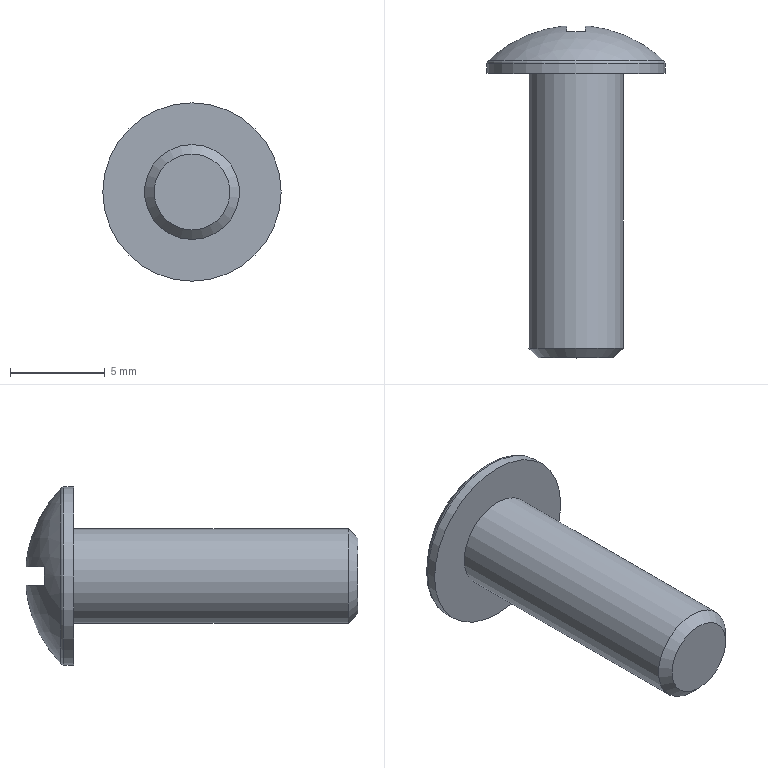Part | STEP file | SD10412 | 1 solid | 24 faces | box 9.4 x 17.503 x 9.4 mm | volume 388.67 mm3 | plane 15 | cylinder 6 | sphere 1 | cone 1 | torus 1 | commonest cylinder face diameters 0.4 x4 5 x1 9.4 x1